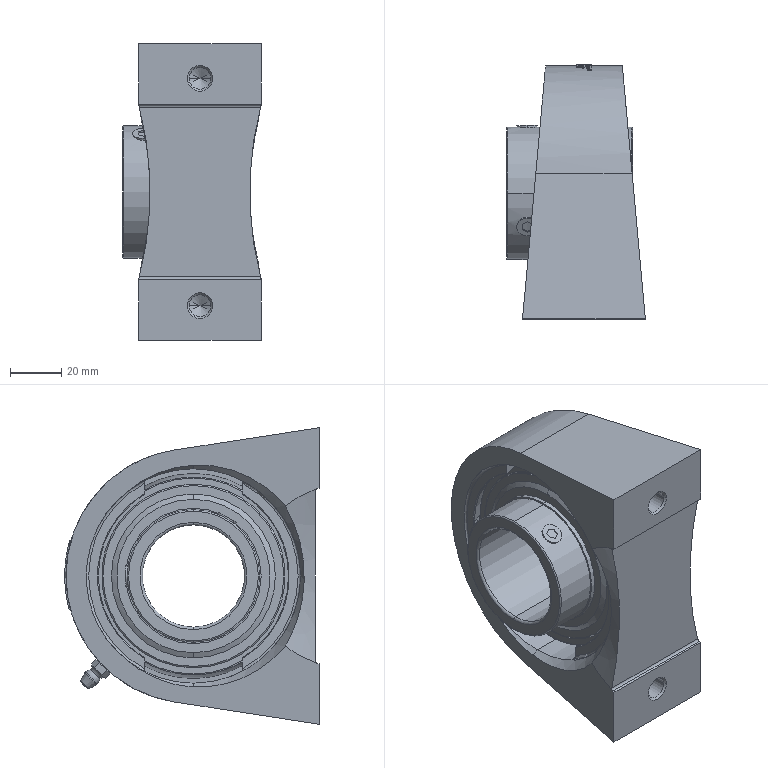Part | SolidWorks | features AEMSimFeature 1 | 12 solids | 436 faces | box 54.2 x 99.5 x 116 mm | volume 238487 mm3 | plane 133 | cylinder 126 | cone 97 | torus 52 | sphere 28 | commonest cylinder face diameters 0.193 x14 0.333 x14 51.8 x14 0.615 x13 0.189 x10 83.871 x6